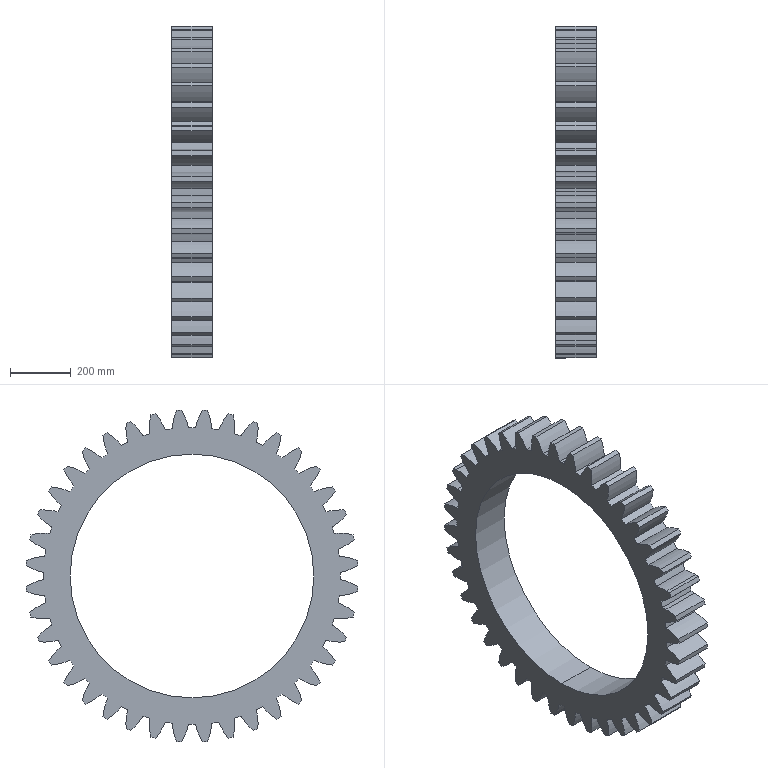Part | SolidWorks | features ICE 2, BaseBody 1, Scale 1 | 1 solid | 169 faces | box 132.6 x 1090 x 1090 mm | volume 44239746 mm3 | cylinder 167 | plane 2 | commonest cylinder face diameters 416 x84 974.999 x41 1092 x40 800 x2